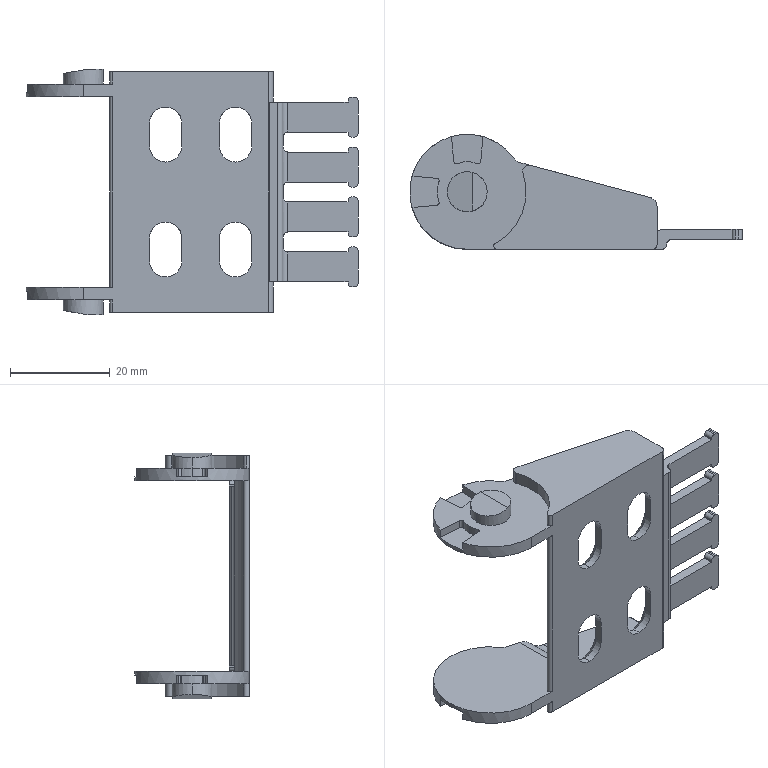Part | SolidWorks | features BaseBody 1 | 1 solid | 184 faces | box 66.5 x 23 x 49.2 mm | volume 8628 mm3 | plane 89 | cylinder 83 | cone 12 | commonest cylinder face diameters 1.5 x16 1 x12 6.5 x12 2 x11 1.2 x6 8 x6